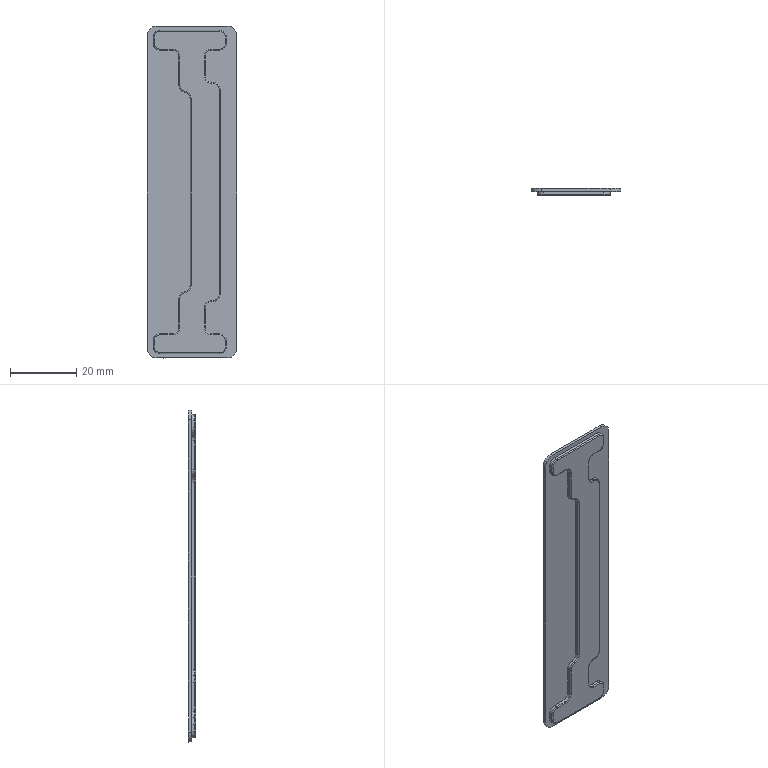Part | SolidWorks | features MoveFace 2, BaseBody 1 | 1 solid | 1417 faces | box 27 x 2.11 x 100 mm | volume 3661 mm3 | plane 1318 | cylinder 79 | spline 20 | commonest cylinder face diameters 6 x33 0.6 x18 3.9 x12 4.1 x8 0.256 x2 0.258 x2